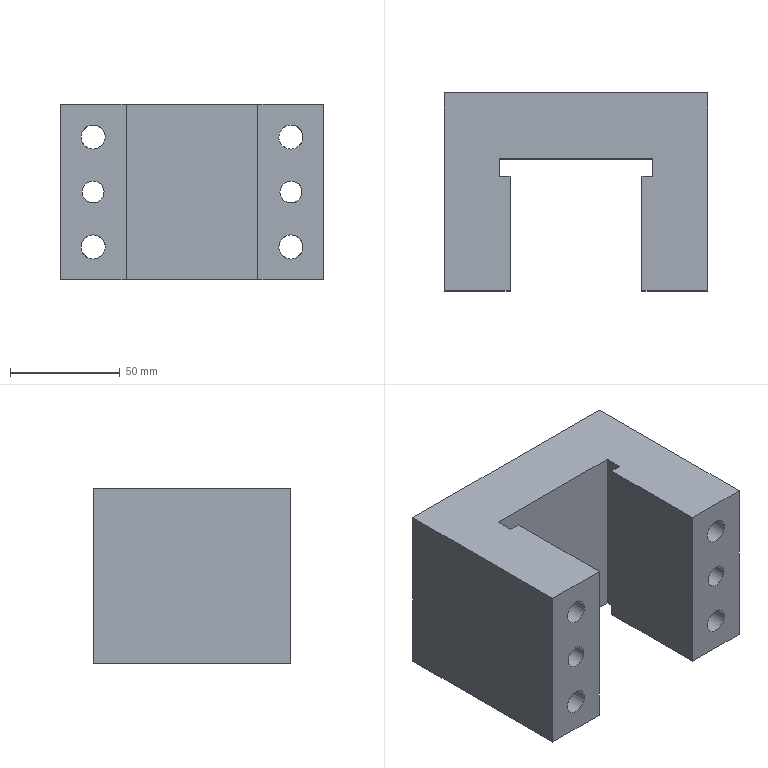Part | STEP file | solid 144 | 1 solid | 32 faces | box 120 x 90 x 80 mm | volume 514851 mm3 | plane 18 | cylinder 10 | cone 4 | commonest cylinder face diameters 11 x4 17.5 x4 10 x2